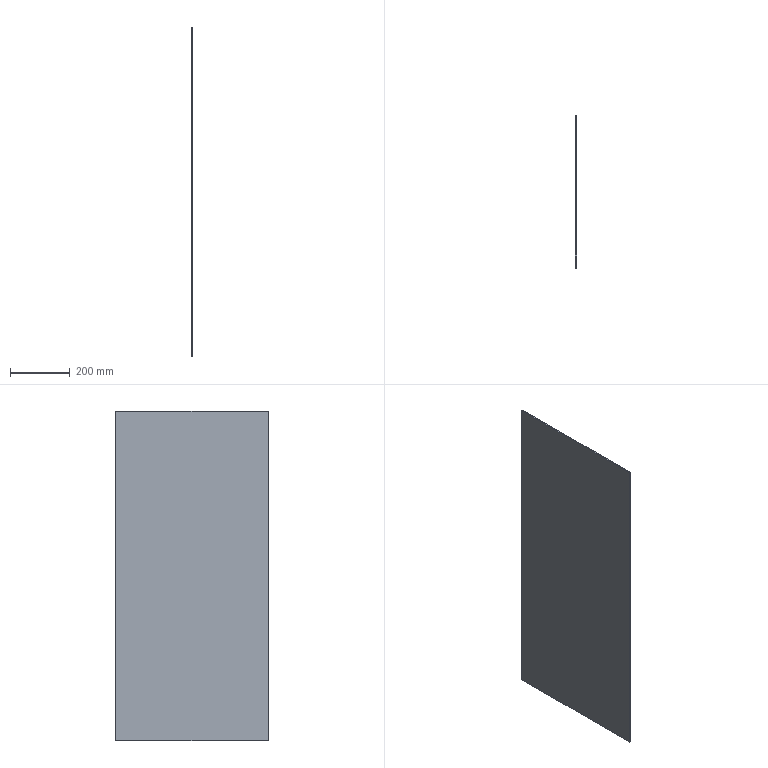Part | STEP file | 1 solid | 6 faces | box 4 x 509 x 1099 mm | volume 2237564 mm3 | plane 6
STEP:
#1=CARTESIAN_POINT('',(0.,0.,0.));
#2=DIRECTION('',(0.,0.,1.));
#3=DIRECTION('',(1.,0.,0.));
#4=AXIS2_PLACEMENT_3D('',#1,#2,#3);
#5=CARTESIAN_POINT('',(761.,4415.3,1218.894));
#6=VERTEX_POINT('',#5);
#7=CARTESIAN_POINT('',(761.,4415.3,119.894));
#8=VERTEX_POINT('',#7);
#9=CARTESIAN_POINT('',(761.,4415.3,1218.894));
#10=DIRECTION('',(0.,0.,-1.));
#11=VECTOR('',#10,1.);
#12=LINE('',#9,#11);
#13=CARTESIAN_POINT('',(761.,4160.8,884.394));
#14=DIRECTION('',(1.,0.,0.));
#15=DIRECTION('',(0.,0.,-1.));
#16=AXIS2_PLACEMENT_3D('',#13,#14,#15);
#17=PLANE('',#16);
#18=CARTESIAN_POINT('',(-334.5,254.5));
#19=DIRECTION('',(1.,0.));
#20=VECTOR('',#19,1.);
#21=LINE('',#18,#20);
#22=(GEOMETRIC_REPRESENTATION_CONTEXT(2)PARAMETRIC_REPRESENTATION_CONTEXT()REPRESENTATION_CONTEXT('',''));
#23=DEFINITIONAL_REPRESENTATION('',(#21),#22);
#24=PCURVE('',#17,#23);
#25=CARTESIAN_POINT('',(761.,4415.3,1648.894));
#26=DIRECTION('',(0.,1.,0.));
#27=DIRECTION('',(0.,0.,1.));
#28=AXIS2_PLACEMENT_3D('',#25,#26,#27);
#29=PLANE('',#28);
#30=CARTESIAN_POINT('',(-430.,0.));
#31=DIRECTION('',(-1.,0.));
#32=VECTOR('',#31,1.);
#33=LINE('',#30,#32);
#34=(GEOMETRIC_REPRESENTATION_CONTEXT(2)PARAMETRIC_REPRESENTATION_CONTEXT()REPRESENTATION_CONTEXT('',''));
#35=DEFINITIONAL_REPRESENTATION('',(#33),#34);
#36=PCURVE('',#29,#35);
#37=SURFACE_CURVE('',#12,(#24,#36),.PCURVE_S1.);
#38=EDGE_CURVE('',#6,#8,#37,.T.);
#39=ORIENTED_EDGE('',*,*,#38,.F.);
#40=CARTESIAN_POINT('',(761.,3906.3,1218.894));
#41=VERTEX_POINT('',#40);
#42=CARTESIAN_POINT('',(761.,3906.3,1218.894));
#43=DIRECTION('',(0.,1.,0.));
#44=VECTOR('',#43,1.);
#45=LINE('',#42,#44);
#46=CARTESIAN_POINT('',(-334.5,-254.5));
#47=DIRECTION('',(0.,1.));
#48=VECTOR('',#47,1.);
#49=LINE('',#46,#48);
#50=(GEOMETRIC_REPRESENTATION_CONTEXT(2)PARAMETRIC_REPRESENTATION_CONTEXT()REPRESENTATION_CONTEXT('',''));
#51=DEFINITIONAL_REPRESENTATION('',(#49),#50);
#52=PCURVE('',#17,#51);
#53=CARTESIAN_POINT('',(761.,3906.3,1218.894));
#54=DIRECTION('',(0.,0.,1.));
#55=DIRECTION('',(0.,-1.,0.));
#56=AXIS2_PLACEMENT_3D('',#53,#54,#55);
#57=PLANE('',#56);
#58=CARTESIAN_POINT('',(0.,0.));
#59=DIRECTION('',(-1.,0.));
#60=VECTOR('',#59,1.);
#61=LINE('',#58,#60);
#62=(GEOMETRIC_REPRESENTATION_CONTEXT(2)PARAMETRIC_REPRESENTATION_CONTEXT()REPRESENTATION_CONTEXT('',''));
#63=DEFINITIONAL_REPRESENTATION('',(#61),#62);
#64=PCURVE('',#57,#63);
#65=SURFACE_CURVE('',#45,(#52,#64),.PCURVE_S1.);
#66=EDGE_CURVE('',#41,#6,#65,.T.);
#67=ORIENTED_EDGE('',*,*,#66,.F.);
#68=CARTESIAN_POINT('',(761.,3906.3,119.894));
#69=VERTEX_POINT('',#68);
#70=CARTESIAN_POINT('',(761.,3906.3,119.894));
#71=DIRECTION('',(0.,0.,1.));
#72=VECTOR('',#71,1.);
#73=LINE('',#70,#72);
#74=CARTESIAN_POINT('',(764.5,-254.5));
#75=DIRECTION('',(-1.,0.));
#76=VECTOR('',#75,1.);
#77=LINE('',#74,#76);
#78=(GEOMETRIC_REPRESENTATION_CONTEXT(2)PARAMETRIC_REPRESENTATION_CONTEXT()REPRESENTATION_CONTEXT('',''));
#79=DEFINITIONAL_REPRESENTATION('',(#77),#78);
#80=PCURVE('',#17,#79);
#81=CARTESIAN_POINT('',(761.,3906.3,119.894));
#82=DIRECTION('',(0.,-1.,0.));
#83=DIRECTION('',(0.,0.,-1.));
#84=AXIS2_PLACEMENT_3D('',#81,#82,#83);
#85=PLANE('',#84);
#86=CARTESIAN_POINT('',(0.,0.));
#87=DIRECTION('',(-1.,0.));
#88=VECTOR('',#87,1.);
#89=LINE('',#86,#88);
#90=(GEOMETRIC_REPRESENTATION_CONTEXT(2)PARAMETRIC_REPRESENTATION_CONTEXT()REPRESENTATION_CONTEXT('',''));
#91=DEFINITIONAL_REPRESENTATION('',(#89),#90);
#92=PCURVE('',#85,#91);
#93=SURFACE_CURVE('',#73,(#80,#92),.PCURVE_S1.);
#94=EDGE_CURVE('',#69,#41,#93,.T.);
#95=ORIENTED_EDGE('',*,*,#94,.F.);
#96=CARTESIAN_POINT('',(761.,4415.3,119.894));
#97=DIRECTION('',(0.,-1.,0.));
#98=VECTOR('',#97,1.);
#99=LINE('',#96,#98);
#100=CARTESIAN_POINT('',(764.5,254.5));
#101=DIRECTION('',(0.,-1.));
#102=VECTOR('',#101,1.);
#103=LINE('',#100,#102);
#104=(GEOMETRIC_REPRESENTATION_CONTEXT(2)PARAMETRIC_REPRESENTATION_CONTEXT()REPRESENTATION_CONTEXT('',''));
#105=DEFINITIONAL_REPRESENTATION('',(#103),#104);
#106=PCURVE('',#17,#105);
#107=CARTESIAN_POINT('',(761.,4415.3,119.894));
#108=DIRECTION('',(0.,0.,-1.));
#109=DIRECTION('',(0.,1.,0.));
#110=AXIS2_PLACEMENT_3D('',#107,#108,#109);
#111=PLANE('',#110);
#112=CARTESIAN_POINT('',(0.,0.));
#113=DIRECTION('',(-1.,0.));
#114=VECTOR('',#113,1.);
#115=LINE('',#112,#114);
#116=(GEOMETRIC_REPRESENTATION_CONTEXT(2)PARAMETRIC_REPRESENTATION_CONTEXT()REPRESENTATION_CONTEXT('',''));
#117=DEFINITIONAL_REPRESENTATION('',(#115),#116);
#118=PCURVE('',#111,#117);
#119=SURFACE_CURVE('',#99,(#106,#118),.PCURVE_S1.);
#120=EDGE_CURVE('',#8,#69,#119,.T.);
#121=ORIENTED_EDGE('',*,*,#120,.F.);
#122=EDGE_LOOP('',(#39,#67,#95,#121));
#123=FACE_BOUND('',#122,.F.);
#124=ADVANCED_FACE('',(#123),#17,.F.);
#125=CARTESIAN_POINT('',(765.,4415.3,119.894));
#126=VERTEX_POINT('',#125);
#127=CARTESIAN_POINT('',(761.,4415.3,119.894));
#128=DIRECTION('',(1.,0.,0.));
#129=VECTOR('',#128,1.);
#130=LINE('',#127,#129);
#131=CARTESIAN_POINT('',(-1529.,0.));
#132=DIRECTION('',(0.,1.));
#133=VECTOR('',#132,1.);
#134=LINE('',#131,#133);
#135=(GEOMETRIC_REPRESENTATION_CONTEXT(2)PARAMETRIC_REPRESENTATION_CONTEXT()REPRESENTATION_CONTEXT('',''));
#136=DEFINITIONAL_REPRESENTATION('',(#134),#135);
#137=PCURVE('',#29,#136);
#138=CARTESIAN_POINT('',(0.,0.));
#139=DIRECTION('',(0.,1.));
#140=VECTOR('',#139,1.);
#141=LINE('',#138,#140);
#142=(GEOMETRIC_REPRESENTATION_CONTEXT(2)PARAMETRIC_REPRESENTATION_CONTEXT()REPRESENTATION_CONTEXT('',''));
#143=DEFINITIONAL_REPRESENTATION('',(#141),#142);
#144=PCURVE('',#111,#143);
#145=SURFACE_CURVE('',#130,(#137,#144),.PCURVE_S1.);
#146=EDGE_CURVE('',#8,#126,#145,.T.);
#147=ORIENTED_EDGE('',*,*,#146,.T.);
#148=CARTESIAN_POINT('',(765.,4415.3,1218.894));
#149=VERTEX_POINT('',#148);
#150=CARTESIAN_POINT('',(765.,4415.3,1218.894));
#151=DIRECTION('',(0.,0.,-1.));
#152=VECTOR('',#151,1.);
#153=LINE('',#150,#152);
#154=CARTESIAN_POINT('',(-430.,4.));
#155=DIRECTION('',(-1.,0.));
#156=VECTOR('',#155,1.);
#157=LINE('',#154,#156);
#158=(GEOMETRIC_REPRESENTATION_CONTEXT(2)PARAMETRIC_REPRESENTATION_CONTEXT()REPRESENTATION_CONTEXT('',''));
#159=DEFINITIONAL_REPRESENTATION('',(#157),#158);
#160=PCURVE('',#29,#159);
#161=CARTESIAN_POINT('',(765.,4160.8,884.394));
#162=DIRECTION('',(1.,0.,0.));
#163=DIRECTION('',(0.,0.,-1.));
#164=AXIS2_PLACEMENT_3D('',#161,#162,#163);
#165=PLANE('',#164);
#166=CARTESIAN_POINT('',(-334.5,254.5));
#167=DIRECTION('',(1.,0.));
#168=VECTOR('',#167,1.);
#169=LINE('',#166,#168);
#170=(GEOMETRIC_REPRESENTATION_CONTEXT(2)PARAMETRIC_REPRESENTATION_CONTEXT()REPRESENTATION_CONTEXT('',''));
#171=DEFINITIONAL_REPRESENTATION('',(#169),#170);
#172=PCURVE('',#165,#171);
#173=SURFACE_CURVE('',#153,(#160,#172),.PCURVE_S1.);
#174=EDGE_CURVE('',#149,#126,#173,.T.);
#175=ORIENTED_EDGE('',*,*,#174,.F.);
#176=CARTESIAN_POINT('',(761.,4415.3,1218.894));
#177=DIRECTION('',(1.,0.,0.));
#178=VECTOR('',#177,1.);
#179=LINE('',#176,#178);
#180=CARTESIAN_POINT('',(-430.,0.));
#181=DIRECTION('',(0.,1.));
#182=VECTOR('',#181,1.);
#183=LINE('',#180,#182);
#184=(GEOMETRIC_REPRESENTATION_CONTEXT(2)PARAMETRIC_REPRESENTATION_CONTEXT()REPRESENTATION_CONTEXT('',''));
#185=DEFINITIONAL_REPRESENTATION('',(#183),#184);
#186=PCURVE('',#29,#185);
#187=CARTESIAN_POINT('',(-509.,0.));
#188=DIRECTION('',(0.,1.));
#189=VECTOR('',#188,1.);
#190=LINE('',#187,#189);
#191=(GEOMETRIC_REPRESENTATION_CONTEXT(2)PARAMETRIC_REPRESENTATION_CONTEXT()REPRESENTATION_CONTEXT('',''));
#192=DEFINITIONAL_REPRESENTATION('',(#190),#191);
#193=PCURVE('',#57,#192);
#194=SURFACE_CURVE('',#179,(#186,#193),.PCURVE_S1.);
#195=EDGE_CURVE('',#6,#149,#194,.T.);
#196=ORIENTED_EDGE('',*,*,#195,.F.);
#197=ORIENTED_EDGE('',*,*,#38,.T.);
#198=EDGE_LOOP('',(#147,#175,#196,#197));
#199=FACE_BOUND('',#198,.F.);
#200=ADVANCED_FACE('',(#199),#29,.T.);
#201=CARTESIAN_POINT('',(765.,3906.3,119.894));
#202=VERTEX_POINT('',#201);
#203=CARTESIAN_POINT('',(761.,3906.3,119.894));
#204=DIRECTION('',(1.,0.,0.));
#205=VECTOR('',#204,1.);
#206=LINE('',#203,#205);
#207=CARTESIAN_POINT('',(-509.,0.));
#208=DIRECTION('',(0.,1.));
#209=VECTOR('',#208,1.);
#210=LINE('',#207,#209);
#211=(GEOMETRIC_REPRESENTATION_CONTEXT(2)PARAMETRIC_REPRESENTATION_CONTEXT()REPRESENTATION_CONTEXT('',''));
#212=DEFINITIONAL_REPRESENTATION('',(#210),#211);
#213=PCURVE('',#111,#212);
#214=CARTESIAN_POINT('',(0.,0.));
#215=DIRECTION('',(0.,1.));
#216=VECTOR('',#215,1.);
#217=LINE('',#214,#216);
#218=(GEOMETRIC_REPRESENTATION_CONTEXT(2)PARAMETRIC_REPRESENTATION_CONTEXT()REPRESENTATION_CONTEXT('',''));
#219=DEFINITIONAL_REPRESENTATION('',(#217),#218);
#220=PCURVE('',#85,#219);
#221=SURFACE_CURVE('',#206,(#213,#220),.PCURVE_S1.);
#222=EDGE_CURVE('',#69,#202,#221,.T.);
#223=ORIENTED_EDGE('',*,*,#222,.T.);
#224=CARTESIAN_POINT('',(765.,4415.3,119.894));
#225=DIRECTION('',(0.,-1.,0.));
#226=VECTOR('',#225,1.);
#227=LINE('',#224,#226);
#228=CARTESIAN_POINT('',(0.,4.));
#229=DIRECTION('',(-1.,0.));
#230=VECTOR('',#229,1.);
#231=LINE('',#228,#230);
#232=(GEOMETRIC_REPRESENTATION_CONTEXT(2)PARAMETRIC_REPRESENTATION_CONTEXT()REPRESENTATION_CONTEXT('',''));
#233=DEFINITIONAL_REPRESENTATION('',(#231),#232);
#234=PCURVE('',#111,#233);
#235=CARTESIAN_POINT('',(764.5,254.5));
#236=DIRECTION('',(0.,-1.));
#237=VECTOR('',#236,1.);
#238=LINE('',#235,#237);
#239=(GEOMETRIC_REPRESENTATION_CONTEXT(2)PARAMETRIC_REPRESENTATION_CONTEXT()REPRESENTATION_CONTEXT('',''));
#240=DEFINITIONAL_REPRESENTATION('',(#238),#239);
#241=PCURVE('',#165,#240);
#242=SURFACE_CURVE('',#227,(#234,#241),.PCURVE_S1.);
#243=EDGE_CURVE('',#126,#202,#242,.T.);
#244=ORIENTED_EDGE('',*,*,#243,.F.);
#245=ORIENTED_EDGE('',*,*,#146,.F.);
#246=ORIENTED_EDGE('',*,*,#120,.T.);
#247=EDGE_LOOP('',(#223,#244,#245,#246));
#248=FACE_BOUND('',#247,.F.);
#249=ADVANCED_FACE('',(#248),#111,.T.);
#250=CARTESIAN_POINT('',(765.,3906.3,1218.894));
#251=VERTEX_POINT('',#250);
#252=CARTESIAN_POINT('',(761.,3906.3,1218.894));
#253=DIRECTION('',(1.,0.,0.));
#254=VECTOR('',#253,1.);
#255=LINE('',#252,#254);
#256=CARTESIAN_POINT('',(-1099.,0.));
#257=DIRECTION('',(0.,1.));
#258=VECTOR('',#257,1.);
#259=LINE('',#256,#258);
#260=(GEOMETRIC_REPRESENTATION_CONTEXT(2)PARAMETRIC_REPRESENTATION_CONTEXT()REPRESENTATION_CONTEXT('',''));
#261=DEFINITIONAL_REPRESENTATION('',(#259),#260);
#262=PCURVE('',#85,#261);
#263=CARTESIAN_POINT('',(0.,0.));
#264=DIRECTION('',(0.,1.));
#265=VECTOR('',#264,1.);
#266=LINE('',#263,#265);
#267=(GEOMETRIC_REPRESENTATION_CONTEXT(2)PARAMETRIC_REPRESENTATION_CONTEXT()REPRESENTATION_CONTEXT('',''));
#268=DEFINITIONAL_REPRESENTATION('',(#266),#267);
#269=PCURVE('',#57,#268);
#270=SURFACE_CURVE('',#255,(#262,#269),.PCURVE_S1.);
#271=EDGE_CURVE('',#41,#251,#270,.T.);
#272=ORIENTED_EDGE('',*,*,#271,.T.);
#273=CARTESIAN_POINT('',(765.,3906.3,119.894));
#274=DIRECTION('',(0.,0.,1.));
#275=VECTOR('',#274,1.);
#276=LINE('',#273,#275);
#277=CARTESIAN_POINT('',(0.,4.));
#278=DIRECTION('',(-1.,0.));
#279=VECTOR('',#278,1.);
#280=LINE('',#277,#279);
#281=(GEOMETRIC_REPRESENTATION_CONTEXT(2)PARAMETRIC_REPRESENTATION_CONTEXT()REPRESENTATION_CONTEXT('',''));
#282=DEFINITIONAL_REPRESENTATION('',(#280),#281);
#283=PCURVE('',#85,#282);
#284=CARTESIAN_POINT('',(764.5,-254.5));
#285=DIRECTION('',(-1.,0.));
#286=VECTOR('',#285,1.);
#287=LINE('',#284,#286);
#288=(GEOMETRIC_REPRESENTATION_CONTEXT(2)PARAMETRIC_REPRESENTATION_CONTEXT()REPRESENTATION_CONTEXT('',''));
#289=DEFINITIONAL_REPRESENTATION('',(#287),#288);
#290=PCURVE('',#165,#289);
#291=SURFACE_CURVE('',#276,(#283,#290),.PCURVE_S1.);
#292=EDGE_CURVE('',#202,#251,#291,.T.);
#293=ORIENTED_EDGE('',*,*,#292,.F.);
#294=ORIENTED_EDGE('',*,*,#222,.F.);
#295=ORIENTED_EDGE('',*,*,#94,.T.);
#296=EDGE_LOOP('',(#272,#293,#294,#295));
#297=FACE_BOUND('',#296,.F.);
#298=ADVANCED_FACE('',(#297),#85,.T.);
#299=ORIENTED_EDGE('',*,*,#195,.T.);
#300=CARTESIAN_POINT('',(765.,3906.3,1218.894));
#301=DIRECTION('',(0.,1.,0.));
#302=VECTOR('',#301,1.);
#303=LINE('',#300,#302);
#304=CARTESIAN_POINT('',(0.,4.));
#305=DIRECTION('',(-1.,0.));
#306=VECTOR('',#305,1.);
#307=LINE('',#304,#306);
#308=(GEOMETRIC_REPRESENTATION_CONTEXT(2)PARAMETRIC_REPRESENTATION_CONTEXT()REPRESENTATION_CONTEXT('',''));
#309=DEFINITIONAL_REPRESENTATION('',(#307),#308);
#310=PCURVE('',#57,#309);
#311=CARTESIAN_POINT('',(-334.5,-254.5));
#312=DIRECTION('',(0.,1.));
#313=VECTOR('',#312,1.);
#314=LINE('',#311,#313);
#315=(GEOMETRIC_REPRESENTATION_CONTEXT(2)PARAMETRIC_REPRESENTATION_CONTEXT()REPRESENTATION_CONTEXT('',''));
#316=DEFINITIONAL_REPRESENTATION('',(#314),#315);
#317=PCURVE('',#165,#316);
#318=SURFACE_CURVE('',#303,(#310,#317),.PCURVE_S1.);
#319=EDGE_CURVE('',#251,#149,#318,.T.);
#320=ORIENTED_EDGE('',*,*,#319,.F.);
#321=ORIENTED_EDGE('',*,*,#271,.F.);
#322=ORIENTED_EDGE('',*,*,#66,.T.);
#323=EDGE_LOOP('',(#299,#320,#321,#322));
#324=FACE_BOUND('',#323,.F.);
#325=ADVANCED_FACE('',(#324),#57,.T.);
#326=ORIENTED_EDGE('',*,*,#292,.T.);
#327=ORIENTED_EDGE('',*,*,#319,.T.);
#328=ORIENTED_EDGE('',*,*,#174,.T.);
#329=ORIENTED_EDGE('',*,*,#243,.T.);
#330=EDGE_LOOP('',(#326,#327,#328,#329));
#331=FACE_BOUND('',#330,.F.);
#332=ADVANCED_FACE('',(#331),#165,.T.);
#333=CLOSED_SHELL('',(#124,#200,#249,#298,#325,#332));
#334=MANIFOLD_SOLID_BREP('',#333);
#335=(LENGTH_UNIT()NAMED_UNIT(*)SI_UNIT(.MILLI.,.METRE.));
#336=UNCERTAINTY_MEASURE_WITH_UNIT(LENGTH_MEASURE(0.0000001),#335,'','');
#337=(NAMED_UNIT(*)PLANE_ANGLE_UNIT()SI_UNIT($,.RADIAN.));
#338=(NAMED_UNIT(*)SI_UNIT($,.STERADIAN.)SOLID_ANGLE_UNIT());
#339=(GEOMETRIC_REPRESENTATION_CONTEXT(3)GLOBAL_UNCERTAINTY_ASSIGNED_CONTEXT((#336))GLOBAL_UNIT_ASSIGNED_CONTEXT((#335,#337,#338))REPRESENTATION_CONTEXT('',''));
#340=ADVANCED_BREP_SHAPE_REPRESENTATION('',(#4,#334),#339);